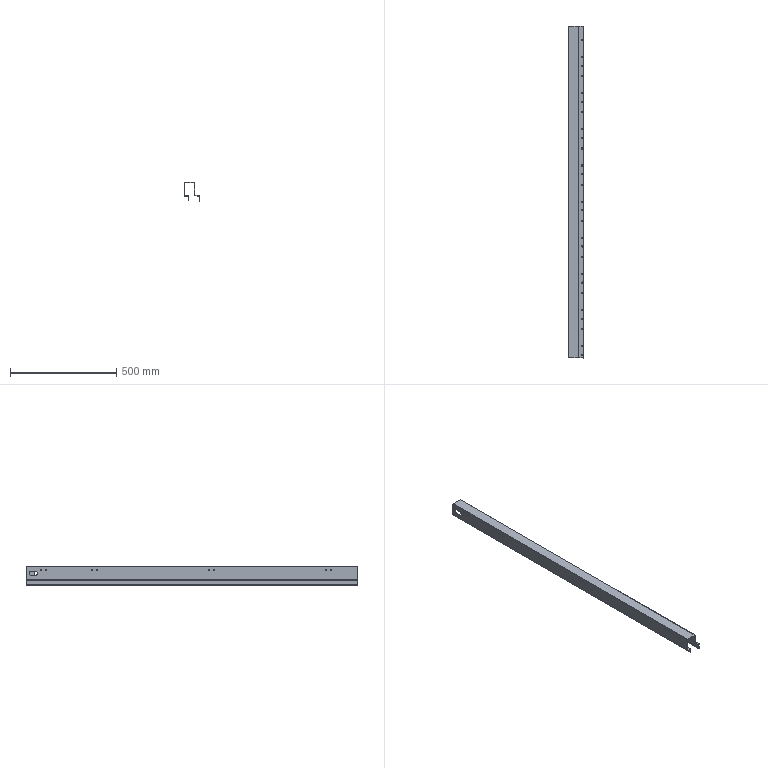Part | SolidWorks | features SplitBody 1 | 1 solid | 378 faces | box 75 x 1562 x 90 mm | volume 569979 mm3 | cylinder 242 | plane 136 | commonest cylinder face diameters 5.5 x70 4.5 x54 10.5 x54 35 x18 6.5 x16 11.5 x16